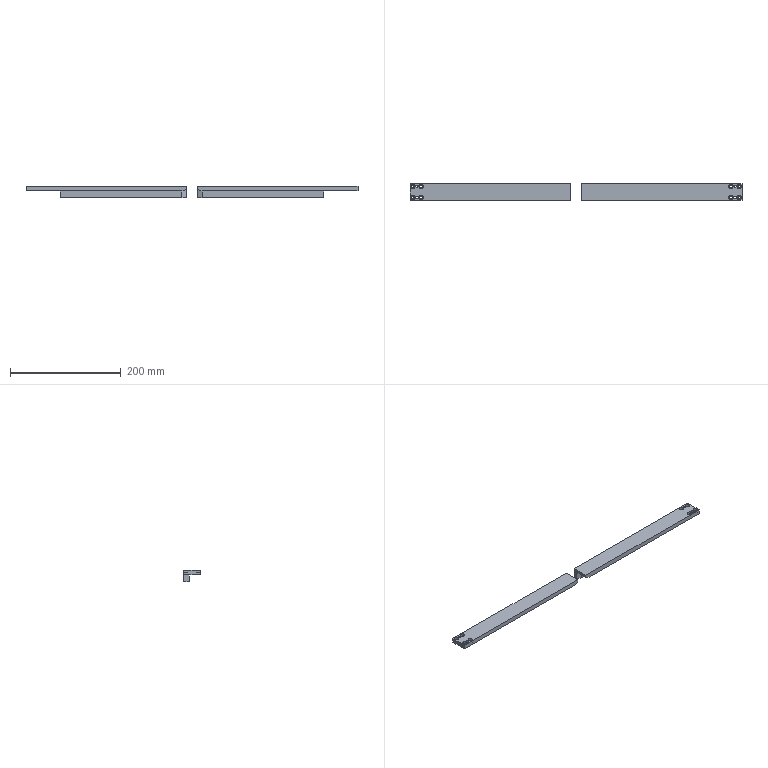NC program | NX | posted with a generic post | part box 600 x 30 x 20 mm
Lines 1 to 414 of 3385:
N10 G17 G21 G94 G90
(FLOOR_WALL_2 , TOOL : D50)
N12 T01 M6
N14 G54
N16 G17 G0 G90 X176. Y0. S6500 M3
N18 G43 Z30. H1
N20 Z3.
N22 G94 G1 Z0. F1250.
N24 X173.
N26 X-173.
N28 X-176.
N30 Z3.
N32 G0 Z30.
N34 M5
(DRILLING_COPY_1_1 , TOOL : D6A45)
N36 T02 M6
N38 G54
N40 G17 G0 G90 X140. Y-10. S3000 M3
N42 G43 Z30. H2
N44 G94 G81 G98 Z-1.6 F200. R3.
N46 X132.5 Y-9.5
N48 X125. Y-10.
N50 Y10.
N52 X132.5
N54 X140.
N56 G80
N58 G0 X140. Y10. Z30.
N60 M5
(DRILLING_COPY_1_COPY_COPY_1_COPY_1_COPY_1 , TOOL : 4.5ZT)
N62 T14 M6
N64 G54
N66 G17 G0 G90 X140. Y10. S2000 M3
N68 G43 Z30. H14
N70 G94 G83 G98 Z-10.852 F120. Q2. R3.
N72 X125.
N74 X140. Y-10.
N76 X125.
N78 G80
N80 G0 X125. Y-10. Z30.
N82 M5
(DRILLING_COPY_1_COPY_COPY_1_COPY_1_COPY_COPY_1 , TOOL : 2.5ZT)
N84 T12 M6
N86 G54
N88 G17 G0 G90 X132.5 Y10. S2000 M3
N90 G43 Z30. H12
N92 G94 G83 G98 Z-10.251 F120. Q2. R3.
N94 Y-9.5
N96 G80
N98 G0 X132.5 Y-9.5 Z30.
N100 M5
(ZLEVEL_PROFILE_1 , TOOL : D10)
N102 T03 M6
N104 G54
N106 G17 G0 G90 X47.703 Y-20.1 S7000 M3
N108 G43 Z30. H3
N110 Z1.5
N112 G94 G1 X0. Z-1. F1000.
N114 X-145. F3000.
N116 G2 X-150.1 Y-15. R5.1
N118 G1 Y15.
N120 G2 X-145. Y20.1 R5.1
N122 G1 X145.
N124 G2 X150.1 Y15. R5.1
N126 G1 Y-15.
N128 G2 X145. Y-20.1 R5.1
N130 G1 X0.
N132 X-0.387 Z-1.007
N134 X-56.903 Z-1.993
N136 X-57.29 Z-2.
N138 X-145.
N140 G2 X-150.1 Y-15. R5.1
N142 G1 Y15.
N144 G2 X-145. Y20.1 R5.1
N146 G1 X145.
N148 G2 X150.1 Y15. R5.1
N150 G1 Y-15.
N152 G2 X145. Y-20.1 R5.1
N154 G1 X0.
N156 X-0.387 Z-2.007
N158 X-56.903 Z-2.993
N160 X-57.29 Z-3.
N162 X-145.
N164 G2 X-150.1 Y-15. R5.1
N166 G1 Y15.
N168 G2 X-145. Y20.1 R5.1
N170 G1 X145.
N172 G2 X150.1 Y15. R5.1
N174 G1 Y-15.
N176 G2 X145. Y-20.1 R5.1
N178 G1 X0.
N180 X-0.387 Z-3.007
N182 X-56.903 Z-3.993
N184 X-57.29 Z-4.
N186 X-145.
N188 G2 X-150.1 Y-15. R5.1
N190 G1 Y15.
N192 G2 X-145. Y20.1 R5.1
N194 G1 X145.
N196 G2 X150.1 Y15. R5.1
N198 G1 Y-15.
N200 G2 X145. Y-20.1 R5.1
N202 G1 X0.
N204 X-0.387 Z-4.007
N206 X-56.903 Z-4.993
N208 X-57.29 Z-5.
N210 X-145.
N212 G2 X-150.1 Y-15. R5.1
N214 G1 Y15.
N216 G2 X-145. Y20.1 R5.1
N218 G1 X145.
N220 G2 X150.1 Y15. R5.1
N222 G1 Y-15.
N224 G2 X145. Y-20.1 R5.1
N226 G1 X0.
N228 X-0.387 Z-5.007
N230 X-56.903 Z-5.993
N232 X-57.29 Z-6.
N234 X-145.
N236 G2 X-150.1 Y-15. R5.1
N238 G1 Y15.
N240 G2 X-145. Y20.1 R5.1
N242 G1 X145.
N244 G2 X150.1 Y15. R5.1
N246 G1 Y-15.
N248 G2 X145. Y-20.1 R5.1
N250 G1 X0.
N252 X-0.387 Z-6.007
N254 X-56.903 Z-6.993
N256 X-57.29 Z-7.
N258 X-145.
N260 G2 X-150.1 Y-15. R5.1
N262 G1 Y15.
N264 G2 X-145. Y20.1 R5.1
N266 G1 X145.
N268 G2 X150.1 Y15. R5.1
N270 G1 Y-15.
N272 G2 X145. Y-20.1 R5.1
N274 G1 X0.
N276 X-0.387 Z-7.007
N278 X-56.903 Z-7.993
N280 X-57.29 Z-8.
N282 X-145.
N284 G2 X-150.1 Y-15. R5.1
N286 G1 Y15.
N288 G2 X-145. Y20.1 R5.1
N290 G1 X145.
N292 G2 X150.1 Y15. R5.1
N294 G1 Y-15.
N296 G2 X145. Y-20.1 R5.1
N298 G1 X0.
N300 X-0.387 Z-8.007
N302 X-56.903 Z-8.993
N304 X-57.29 Z-9.
N306 X-145.
N308 G2 X-150.1 Y-15. R5.1
N310 G1 Y15.
N312 G2 X-145. Y20.1 R5.1
N314 G1 X145.
N316 G2 X150.1 Y15. R5.1
N318 G1 Y-15.
N320 G2 X145. Y-20.1 R5.1
N322 G1 X0.
N324 X-0.387 Z-9.007
N326 X-56.903 Z-9.993
N328 X-57.29 Z-10.
N330 X-145.
N332 G2 X-150.1 Y-15. R5.1
N334 G1 Y15.
N336 G2 X-145. Y20.1 R5.1
N338 G1 X145.
N340 G2 X150.1 Y15. R5.1
N342 G1 Y-15.
N344 G2 X145. Y-20.1 R5.1
N346 G1 X0.
N348 X-0.387 Z-10.007
N350 X-56.903 Z-10.993
N352 X-57.29 Z-11.
N354 X-145.
N356 G2 X-150.1 Y-15. R5.1
N358 G1 Y15.
N360 G2 X-145. Y20.1 R5.1
N362 G1 X145.
N364 G2 X150.1 Y15. R5.1
N366 G1 Y-15.
N368 G2 X145. Y-20.1 R5.1
N370 G1 X0.
N372 X-0.387 Z-11.007
N374 X-56.903 Z-11.993
N376 X-57.29 Z-12.
N378 X-145.
N380 G2 X-150.1 Y-15. R5.1
N382 G1 Y15.
N384 G2 X-145. Y20.1 R5.1
N386 G1 X145.
N388 G2 X150.1 Y15. R5.1
N390 G1 Y-15.
N392 G2 X145. Y-20.1 R5.1
N394 G1 X0.
N396 X-0.387 Z-12.007
N398 X-56.903 Z-12.993
N400 X-57.29 Z-13.
N402 X-145.
N404 G2 X-150.1 Y-15. R5.1
N406 G1 Y15.
N408 G2 X-145. Y20.1 R5.1
N410 G1 X145.
N412 G2 X150.1 Y15. R5.1
N414 G1 Y-15.
N416 G2 X145. Y-20.1 R5.1
N418 G1 X0.
N420 X-0.387 Z-13.007
N422 X-56.903 Z-13.993
N424 X-57.29 Z-14.
N426 X-145.
N428 G2 X-150.1 Y-15. R5.1
N430 G1 Y15.
N432 G2 X-145. Y20.1 R5.1
N434 G1 X145.
N436 G2 X150.1 Y15. R5.1
N438 G1 Y-15.
N440 G2 X145. Y-20.1 R5.1
N442 G1 X0.
N444 X-0.387 Z-14.007
N446 X-56.903 Z-14.993
N448 X-57.29 Z-15.
N450 X-145.
N452 G2 X-150.1 Y-15. R5.1
N454 G1 Y15.
N456 G2 X-145. Y20.1 R5.1
N458 G1 X145.
N460 G2 X150.1 Y15. R5.1
N462 G1 Y-15.
N464 G2 X145. Y-20.1 R5.1
N466 G1 X0.
N468 X-0.387 Z-15.007
N470 X-56.903 Z-15.993
N472 X-57.29 Z-16.
N474 X-145.
N476 G2 X-150.1 Y-15. R5.1
N478 G1 Y15.
N480 G2 X-145. Y20.1 R5.1
N482 G1 X145.
N484 G2 X150.1 Y15. R5.1
N486 G1 Y-15.
N488 G2 X145. Y-20.1 R5.1
N490 G1 X0.
N492 X-0.387 Z-16.007
N494 X-56.903 Z-16.993
N496 X-57.29 Z-17.
N498 X-145.
N500 G2 X-150.1 Y-15. R5.1
N502 G1 Y15.
N504 G2 X-145. Y20.1 R5.1
N506 G1 X145.
N508 G2 X150.1 Y15. R5.1
N510 G1 Y-15.
N512 G2 X145. Y-20.1 R5.1
N514 G1 X0.
N516 X-0.387 Z-17.007
N518 X-56.903 Z-17.993
N520 X-57.29 Z-18.
N522 X-145.
N524 G2 X-150.1 Y-15. R5.1
N526 G1 Y15.
N528 G2 X-145. Y20.1 R5.1
N530 G1 X145.
N532 G2 X150.1 Y15. R5.1
N534 G1 Y-15.
N536 G2 X145. Y-20.1 R5.1
N538 G1 X0.
N540 X-0.387 Z-18.007
N542 X-56.903 Z-18.993
N544 X-57.29 Z-19.
N546 X-145.
N548 G2 X-150.1 Y-15. R5.1
N550 G1 Y15.
N552 G2 X-145. Y20.1 R5.1
N554 G1 X145.
N556 G2 X150.1 Y15. R5.1
N558 G1 Y-15.
N560 G2 X145. Y-20.1 R5.1
N562 G1 X0.
N564 X-0.387 Z-19.007
N566 X-56.903 Z-19.993
N568 X-57.29 Z-20.
N570 X-145.
N572 G2 X-150.1 Y-15. R5.1
N574 G1 Y15.
N576 G2 X-145. Y20.1 R5.1
N578 G1 X145.
N580 G2 X150.1 Y15. R5.1
N582 G1 Y-15.
N584 G2 X145. Y-20.1 R5.1
N586 G1 X-57.29
N588 Z-18.5
N590 G0 Z30.
N592 M5
(ZLEVEL_PROFILE_COPY_COPY_1_COPY_COPY_COPY_1_1 , TOOL : D10JING)
N594 T04 M6
N596 G54
N598 G17 G0 G90 X146.096 Y-20.899 S7000 M3
N600 G43 Z30. H4
N602 Z-20.
N604 G94 G1 X145.866 Y-20.5 F1000.
N606 G3 X145. Y-20. R1.
N608 G1 X-145.
N610 G2 X-150. Y-15. R5.
N612 G1 Y15.
N614 G2 X-145. Y20. R5.
N616 G1 X145.
N618 G2 X150. Y15. R5.
N620 G1 Y-15.
N622 G2 X145. Y-20. R5.
N624 G3 X144.134 Y-20.5 R1.
N626 G1 X143.845 Y-21.
N628 G0 Z30.
N630 M5
(HOLE_MILLING_1_1 , TOOL : D6)
N632 T08 M6
N634 G54
N636 G17 G0 G90 X140. Y10. S7000 M3
N638 G43 Z30. H8
N640 Z0.5
N642 G94 G3 X139.5 Y10.5 R0.5 F1500.
N644 X139. Y10. R0.5
N646 X139. Y10. Z0. I1. J0.
N648 X139. Y10. Z-0.5 I1. J0.
N650 X139. Y10. Z-1. I1. J0.
N652 X139. Y10. Z-1.5 I1. J0.
N654 X139. Y10. Z-2. I1. J0.
N656 X139. Y10. Z-2.5 I1. J0.
N658 X139. Y10. Z-3. I1. J0.
N660 X139. Y10. Z-3.5 I1. J0.
N662 X139. Y10. Z-4. I1. J0.
N664 X139.691 Y10.951 Z-4.4 R-1.
N666 X139.049 Y9.691 R1.
N668 X139.691 Y10.951 R-1.
N670 X139.37 Y10.321 R0.5
N672 X140. Y10. R0.5
N674 G0 Z30.
N676 X125.
N678 Z0.5
N680 G3 X124.5 Y10.5 R0.5
N682 X124. Y10. R0.5
N684 X124. Y10. Z0. I1. J0.
N686 X124. Y10. Z-0.5 I1. J0.
N688 X124. Y10. Z-1. I1. J0.
N690 X124. Y10. Z-1.5 I1. J0.
N692 X124. Y10. Z-2. I1. J0.
N694 X124. Y10. Z-2.5 I1. J0.
N696 X124. Y10. Z-3. I1. J0.
N698 X124. Y10. Z-3.5 I1. J0.
N700 X124. Y10. Z-4. I1. J0.
N702 X124.691 Y10.951 Z-4.4 R-1.
N704 X124.049 Y9.691 R1.
N706 X124.691 Y10.951 R-1.
N708 X124.37 Y10.321 R0.5
N710 X125. Y10. R0.5
N712 G0 Z30.
N714 Y-10.
N716 Z0.5
N718 G3 X124.5 Y-9.5 R0.5
N720 X124. Y-10. R0.5
N722 X124. Y-10. Z0. I1. J0.
N724 X124. Y-10. Z-0.5 I1. J0.
N726 X124. Y-10. Z-1. I1. J0.
N728 X124. Y-10. Z-1.5 I1. J0.
N730 X124. Y-10. Z-2. I1. J0.
N732 X124. Y-10. Z-2.5 I1. J0.
N734 X124. Y-10. Z-3. I1. J0.
N736 X124. Y-10. Z-3.5 I1. J0.
N738 X124. Y-10. Z-4. I1. J0.
N740 X124.691 Y-9.049 Z-4.4 R-1.
N742 X124.049 Y-10.309 R1.
N744 X124.691 Y-9.049 R-1.
N746 X124.37 Y-9.679 R0.5
N748 X125. Y-10. R0.5
N750 G0 Z30.
N752 X140.
N754 Z0.5
N756 G3 X139.5 Y-9.5 R0.5
N758 X139. Y-10. R0.5
N760 X139. Y-10. Z0. I1. J0.
N762 X139. Y-10. Z-0.5 I1. J0.
N764 X139. Y-10. Z-1. I1. J0.
N766 X139. Y-10. Z-1.5 I1. J0.
N768 X139. Y-10. Z-2. I1. J0.
N770 X139. Y-10. Z-2.5 I1. J0.
N772 X139. Y-10. Z-3. I1. J0.
N774 X139. Y-10. Z-3.5 I1. J0.
N776 X139. Y-10. Z-4. I1. J0.
N778 X139.691 Y-9.049 Z-4.4 R-1.
N780 X139.049 Y-10.309 R1.
N782 X139.691 Y-9.049 R-1.
N784 X139.37 Y-9.679 R0.5
N786 X140. Y-10. R0.5
N788 G0 Z30.
N790 M5